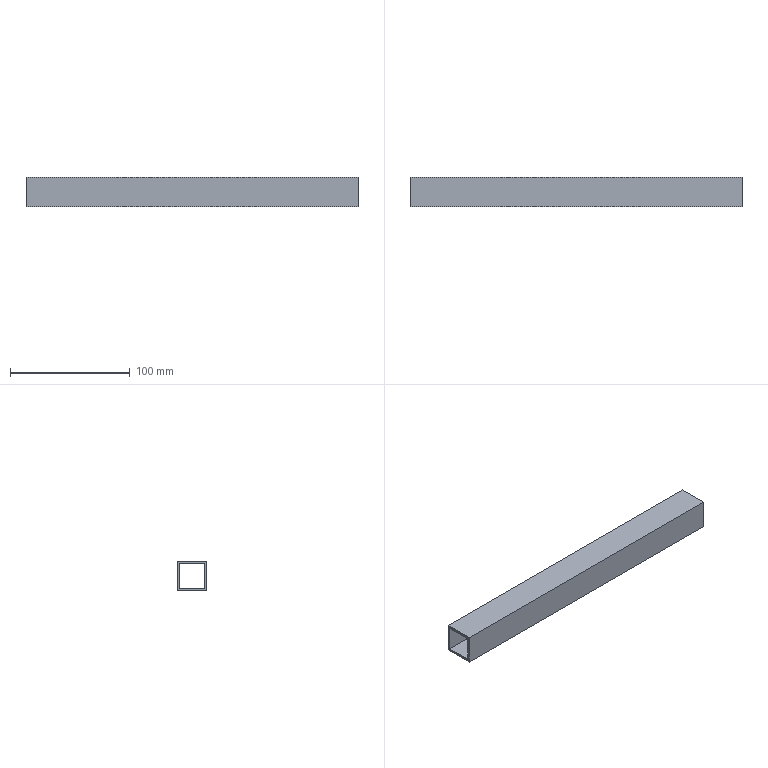Part | NX | features solid 2 | 1 solid | 10 faces | box 277.5 x 25 x 25 mm | volume 51060 mm3 | plane 10
STEP:
#1=CARTESIAN_POINT('',(325.,372.5,35.));
#2=VERTEX_POINT('',#1);
#3=CARTESIAN_POINT('',(325.,372.5,10.));
#4=VERTEX_POINT('',#3);
#5=CARTESIAN_POINT('',(325.,372.5,15.));
#6=DIRECTION('',(0.,0.,-1.));
#7=VECTOR('',#6,1000.);
#8=LINE('',#5,#7);
#9=EDGE_CURVE('',#2,#4,#8,.T.);
#10=ORIENTED_EDGE('',*,*,#9,.T.);
#11=CARTESIAN_POINT('',(47.5,372.5,10.));
#12=VERTEX_POINT('',#11);
#13=CARTESIAN_POINT('',(137.5,372.5,10.));
#14=DIRECTION('',(-1.,0.,0.));
#15=VECTOR('',#14,1000.);
#16=LINE('',#13,#15);
#17=EDGE_CURVE('',#12,#4,#16,.F.);
#18=ORIENTED_EDGE('',*,*,#17,.F.);
#19=CARTESIAN_POINT('',(47.5,372.5,35.));
#20=VERTEX_POINT('',#19);
#21=CARTESIAN_POINT('',(47.5,372.5,15.));
#22=DIRECTION('',(0.,0.,-1.));
#23=VECTOR('',#22,1000.);
#24=LINE('',#21,#23);
#25=EDGE_CURVE('',#12,#20,#24,.F.);
#26=ORIENTED_EDGE('',*,*,#25,.T.);
#27=CARTESIAN_POINT('',(415.,372.5,35.));
#28=DIRECTION('',(-1.,0.,0.));
#29=VECTOR('',#28,1000.);
#30=LINE('',#27,#29);
#31=EDGE_CURVE('',#20,#2,#30,.F.);
#32=ORIENTED_EDGE('',*,*,#31,.T.);
#33=EDGE_LOOP('',(#10,#18,#26,#32));
#34=FACE_BOUND('',#33,.T.);
#35=CARTESIAN_POINT('',(137.5,372.5,15.));
#36=DIRECTION('',(0.,-1.,0.));
#37=DIRECTION('',(0.,0.,-1.));
#38=AXIS2_PLACEMENT_3D('',#35,#36,#37);
#39=PLANE('',#38);
#40=ADVANCED_FACE('',(#34),#39,.F.);
#41=CARTESIAN_POINT('',(47.5,347.5,35.));
#42=VERTEX_POINT('',#41);
#43=CARTESIAN_POINT('',(325.,347.5,35.));
#44=VERTEX_POINT('',#43);
#45=CARTESIAN_POINT('',(415.,347.5,35.));
#46=DIRECTION('',(-1.,0.,0.));
#47=VECTOR('',#46,1000.);
#48=LINE('',#45,#47);
#49=EDGE_CURVE('',#42,#44,#48,.F.);
#50=ORIENTED_EDGE('',*,*,#49,.F.);
#51=CARTESIAN_POINT('',(47.5,347.5,10.));
#52=VERTEX_POINT('',#51);
#53=CARTESIAN_POINT('',(47.5,347.5,15.));
#54=DIRECTION('',(0.,0.,-1.));
#55=VECTOR('',#54,1000.);
#56=LINE('',#53,#55);
#57=EDGE_CURVE('',#52,#42,#56,.F.);
#58=ORIENTED_EDGE('',*,*,#57,.F.);
#59=CARTESIAN_POINT('',(325.,347.5,10.));
#60=VERTEX_POINT('',#59);
#61=CARTESIAN_POINT('',(137.5,347.5,10.));
#62=DIRECTION('',(-1.,0.,0.));
#63=VECTOR('',#62,1000.);
#64=LINE('',#61,#63);
#65=EDGE_CURVE('',#52,#60,#64,.F.);
#66=ORIENTED_EDGE('',*,*,#65,.T.);
#67=CARTESIAN_POINT('',(325.,347.5,15.));
#68=DIRECTION('',(0.,0.,-1.));
#69=VECTOR('',#68,1000.);
#70=LINE('',#67,#69);
#71=EDGE_CURVE('',#44,#60,#70,.T.);
#72=ORIENTED_EDGE('',*,*,#71,.F.);
#73=EDGE_LOOP('',(#50,#58,#66,#72));
#74=FACE_BOUND('',#73,.T.);
#75=CARTESIAN_POINT('',(137.5,347.5,15.));
#76=DIRECTION('',(0.,-1.,0.));
#77=DIRECTION('',(0.,0.,-1.));
#78=AXIS2_PLACEMENT_3D('',#75,#76,#77);
#79=PLANE('',#78);
#80=ADVANCED_FACE('',(#74),#79,.T.);
#81=CARTESIAN_POINT('',(325.,595.,35.));
#82=DIRECTION('',(0.,-1.,0.));
#83=VECTOR('',#82,1000.);
#84=LINE('',#81,#83);
#85=EDGE_CURVE('',#44,#2,#84,.F.);
#86=ORIENTED_EDGE('',*,*,#85,.T.);
#87=ORIENTED_EDGE('',*,*,#31,.F.);
#88=CARTESIAN_POINT('',(47.5,225.,35.));
#89=DIRECTION('',(0.,-1.,0.));
#90=VECTOR('',#89,1000.);
#91=LINE('',#88,#90);
#92=EDGE_CURVE('',#20,#42,#91,.T.);
#93=ORIENTED_EDGE('',*,*,#92,.T.);
#94=ORIENTED_EDGE('',*,*,#49,.T.);
#95=EDGE_LOOP('',(#86,#87,#93,#94));
#96=FACE_BOUND('',#95,.T.);
#97=CARTESIAN_POINT('',(415.,595.,35.));
#98=DIRECTION('',(0.,0.,1.));
#99=DIRECTION('',(0.,-1.,0.));
#100=AXIS2_PLACEMENT_3D('',#97,#98,#99);
#101=PLANE('',#100);
#102=ADVANCED_FACE('',(#96),#101,.T.);
#103=CARTESIAN_POINT('',(325.,-45.,10.));
#104=DIRECTION('',(0.,1.,0.));
#105=VECTOR('',#104,1000.);
#106=LINE('',#103,#105);
#107=EDGE_CURVE('',#4,#60,#106,.F.);
#108=ORIENTED_EDGE('',*,*,#107,.T.);
#109=ORIENTED_EDGE('',*,*,#65,.F.);
#110=CARTESIAN_POINT('',(47.5,-45.,10.));
#111=DIRECTION('',(0.,-1.,0.));
#112=VECTOR('',#111,1000.);
#113=LINE('',#110,#112);
#114=EDGE_CURVE('',#12,#52,#113,.T.);
#115=ORIENTED_EDGE('',*,*,#114,.F.);
#116=ORIENTED_EDGE('',*,*,#17,.T.);
#117=EDGE_LOOP('',(#108,#109,#115,#116));
#118=FACE_BOUND('',#117,.T.);
#119=CARTESIAN_POINT('',(372.5,-45.,10.));
#120=DIRECTION('',(0.,0.,-1.));
#121=DIRECTION('',(-1.,0.,0.));
#122=AXIS2_PLACEMENT_3D('',#119,#120,#121);
#123=PLANE('',#122);
#124=ADVANCED_FACE('',(#118),#123,.T.);
#125=ORIENTED_EDGE('',*,*,#92,.F.);
#126=ORIENTED_EDGE('',*,*,#25,.F.);
#127=ORIENTED_EDGE('',*,*,#114,.T.);
#128=ORIENTED_EDGE('',*,*,#57,.T.);
#129=EDGE_LOOP('',(#125,#126,#127,#128));
#130=FACE_BOUND('',#129,.T.);
#131=CARTESIAN_POINT('',(47.5,370.5,33.));
#132=VERTEX_POINT('',#131);
#133=CARTESIAN_POINT('',(47.5,349.5,33.));
#134=VERTEX_POINT('',#133);
#135=CARTESIAN_POINT('',(47.5,225.,33.));
#136=DIRECTION('',(0.,1.,0.));
#137=VECTOR('',#136,1000.);
#138=LINE('',#135,#137);
#139=EDGE_CURVE('',#132,#134,#138,.F.);
#140=ORIENTED_EDGE('',*,*,#139,.T.);
#141=CARTESIAN_POINT('',(47.5,349.5,12.));
#142=VERTEX_POINT('',#141);
#143=CARTESIAN_POINT('',(47.5,349.5,15.));
#144=DIRECTION('',(0.,0.,-1.));
#145=VECTOR('',#144,1000.);
#146=LINE('',#143,#145);
#147=EDGE_CURVE('',#142,#134,#146,.F.);
#148=ORIENTED_EDGE('',*,*,#147,.F.);
#149=CARTESIAN_POINT('',(47.5,370.5,12.));
#150=VERTEX_POINT('',#149);
#151=CARTESIAN_POINT('',(47.5,225.,12.));
#152=DIRECTION('',(0.,1.,0.));
#153=VECTOR('',#152,1000.);
#154=LINE('',#151,#153);
#155=EDGE_CURVE('',#150,#142,#154,.F.);
#156=ORIENTED_EDGE('',*,*,#155,.F.);
#157=CARTESIAN_POINT('',(47.5,370.5,15.));
#158=DIRECTION('',(0.,0.,-1.));
#159=VECTOR('',#158,1000.);
#160=LINE('',#157,#159);
#161=EDGE_CURVE('',#150,#132,#160,.F.);
#162=ORIENTED_EDGE('',*,*,#161,.T.);
#163=EDGE_LOOP('',(#140,#148,#156,#162));
#164=FACE_BOUND('',#163,.T.);
#165=CARTESIAN_POINT('',(47.5,225.,15.));
#166=DIRECTION('',(-1.,0.,0.));
#167=DIRECTION('',(0.,0.,1.));
#168=AXIS2_PLACEMENT_3D('',#165,#166,#167);
#169=PLANE('',#168);
#170=ADVANCED_FACE('',(#130,#164),#169,.T.);
#171=CARTESIAN_POINT('',(325.,370.5,33.));
#172=VERTEX_POINT('',#171);
#173=CARTESIAN_POINT('',(415.,370.5,33.));
#174=DIRECTION('',(-1.,0.,0.));
#175=VECTOR('',#174,1000.);
#176=LINE('',#173,#175);
#177=EDGE_CURVE('',#132,#172,#176,.F.);
#178=ORIENTED_EDGE('',*,*,#177,.F.);
#179=ORIENTED_EDGE('',*,*,#161,.F.);
#180=CARTESIAN_POINT('',(325.,370.5,12.));
#181=VERTEX_POINT('',#180);
#182=CARTESIAN_POINT('',(137.5,370.5,12.));
#183=DIRECTION('',(-1.,0.,0.));
#184=VECTOR('',#183,1000.);
#185=LINE('',#182,#184);
#186=EDGE_CURVE('',#150,#181,#185,.F.);
#187=ORIENTED_EDGE('',*,*,#186,.T.);
#188=CARTESIAN_POINT('',(325.,370.5,15.));
#189=DIRECTION('',(0.,0.,-1.));
#190=VECTOR('',#189,1000.);
#191=LINE('',#188,#190);
#192=EDGE_CURVE('',#172,#181,#191,.T.);
#193=ORIENTED_EDGE('',*,*,#192,.F.);
#194=EDGE_LOOP('',(#178,#179,#187,#193));
#195=FACE_BOUND('',#194,.T.);
#196=CARTESIAN_POINT('',(137.5,370.5,15.));
#197=DIRECTION('',(0.,-1.,0.));
#198=DIRECTION('',(0.,0.,-1.));
#199=AXIS2_PLACEMENT_3D('',#196,#197,#198);
#200=PLANE('',#199);
#201=ADVANCED_FACE('',(#195),#200,.T.);
#202=CARTESIAN_POINT('',(325.,349.5,33.));
#203=VERTEX_POINT('',#202);
#204=CARTESIAN_POINT('',(325.,349.5,12.));
#205=VERTEX_POINT('',#204);
#206=CARTESIAN_POINT('',(325.,349.5,15.));
#207=DIRECTION('',(0.,0.,-1.));
#208=VECTOR('',#207,1000.);
#209=LINE('',#206,#208);
#210=EDGE_CURVE('',#203,#205,#209,.T.);
#211=ORIENTED_EDGE('',*,*,#210,.T.);
#212=CARTESIAN_POINT('',(137.5,349.5,12.));
#213=DIRECTION('',(-1.,0.,0.));
#214=VECTOR('',#213,1000.);
#215=LINE('',#212,#214);
#216=EDGE_CURVE('',#142,#205,#215,.F.);
#217=ORIENTED_EDGE('',*,*,#216,.F.);
#218=ORIENTED_EDGE('',*,*,#147,.T.);
#219=CARTESIAN_POINT('',(415.,349.5,33.));
#220=DIRECTION('',(-1.,0.,0.));
#221=VECTOR('',#220,1000.);
#222=LINE('',#219,#221);
#223=EDGE_CURVE('',#134,#203,#222,.F.);
#224=ORIENTED_EDGE('',*,*,#223,.T.);
#225=EDGE_LOOP('',(#211,#217,#218,#224));
#226=FACE_BOUND('',#225,.T.);
#227=CARTESIAN_POINT('',(137.5,349.5,15.));
#228=DIRECTION('',(0.,-1.,0.));
#229=DIRECTION('',(0.,0.,-1.));
#230=AXIS2_PLACEMENT_3D('',#227,#228,#229);
#231=PLANE('',#230);
#232=ADVANCED_FACE('',(#226),#231,.F.);
#233=ORIENTED_EDGE('',*,*,#223,.F.);
#234=ORIENTED_EDGE('',*,*,#139,.F.);
#235=ORIENTED_EDGE('',*,*,#177,.T.);
#236=CARTESIAN_POINT('',(325.,595.,33.));
#237=DIRECTION('',(0.,-1.,0.));
#238=VECTOR('',#237,1000.);
#239=LINE('',#236,#238);
#240=EDGE_CURVE('',#203,#172,#239,.F.);
#241=ORIENTED_EDGE('',*,*,#240,.F.);
#242=EDGE_LOOP('',(#233,#234,#235,#241));
#243=FACE_BOUND('',#242,.T.);
#244=CARTESIAN_POINT('',(415.,595.,33.));
#245=DIRECTION('',(0.,0.,1.));
#246=DIRECTION('',(0.,-1.,0.));
#247=AXIS2_PLACEMENT_3D('',#244,#245,#246);
#248=PLANE('',#247);
#249=ADVANCED_FACE('',(#243),#248,.F.);
#250=ORIENTED_EDGE('',*,*,#186,.F.);
#251=ORIENTED_EDGE('',*,*,#155,.T.);
#252=ORIENTED_EDGE('',*,*,#216,.T.);
#253=CARTESIAN_POINT('',(325.,-45.,12.));
#254=DIRECTION('',(0.,1.,0.));
#255=VECTOR('',#254,1000.);
#256=LINE('',#253,#255);
#257=EDGE_CURVE('',#181,#205,#256,.F.);
#258=ORIENTED_EDGE('',*,*,#257,.F.);
#259=EDGE_LOOP('',(#250,#251,#252,#258));
#260=FACE_BOUND('',#259,.T.);
#261=CARTESIAN_POINT('',(372.5,-45.,12.));
#262=DIRECTION('',(0.,0.,-1.));
#263=DIRECTION('',(-1.,0.,0.));
#264=AXIS2_PLACEMENT_3D('',#261,#262,#263);
#265=PLANE('',#264);
#266=ADVANCED_FACE('',(#260),#265,.F.);
#267=ORIENTED_EDGE('',*,*,#71,.T.);
#268=ORIENTED_EDGE('',*,*,#107,.F.);
#269=ORIENTED_EDGE('',*,*,#9,.F.);
#270=ORIENTED_EDGE('',*,*,#85,.F.);
#271=EDGE_LOOP('',(#267,#268,#269,#270));
#272=FACE_BOUND('',#271,.T.);
#273=ORIENTED_EDGE('',*,*,#240,.T.);
#274=ORIENTED_EDGE('',*,*,#192,.T.);
#275=ORIENTED_EDGE('',*,*,#257,.T.);
#276=ORIENTED_EDGE('',*,*,#210,.F.);
#277=EDGE_LOOP('',(#273,#274,#275,#276));
#278=FACE_BOUND('',#277,.T.);
#279=CARTESIAN_POINT('',(325.,-537.5,20.));
#280=DIRECTION('',(1.,0.,0.));
#281=DIRECTION('',(0.,0.,-1.));
#282=AXIS2_PLACEMENT_3D('',#279,#280,#281);
#283=PLANE('',#282);
#284=ADVANCED_FACE('',(#272,#278),#283,.T.);
#285=CLOSED_SHELL('',(#40,#80,#102,#124,#170,#201,#232,#249,#266,#284));
#286=MANIFOLD_SOLID_BREP('',#285);
#287=(LENGTH_UNIT()NAMED_UNIT(*)SI_UNIT(.MILLI.,.METRE.));
#288=UNCERTAINTY_MEASURE_WITH_UNIT(LENGTH_MEASURE(0.00001),#287,'','');
#289=(NAMED_UNIT(*)PLANE_ANGLE_UNIT()SI_UNIT($,.RADIAN.));
#290=(NAMED_UNIT(*)SI_UNIT($,.STERADIAN.)SOLID_ANGLE_UNIT());
#291=(GEOMETRIC_REPRESENTATION_CONTEXT(3)GLOBAL_UNCERTAINTY_ASSIGNED_CONTEXT((#288))GLOBAL_UNIT_ASSIGNED_CONTEXT((#287,#289,#290))REPRESENTATION_CONTEXT('',''));
#292=ADVANCED_BREP_SHAPE_REPRESENTATION('',(#286),#291);